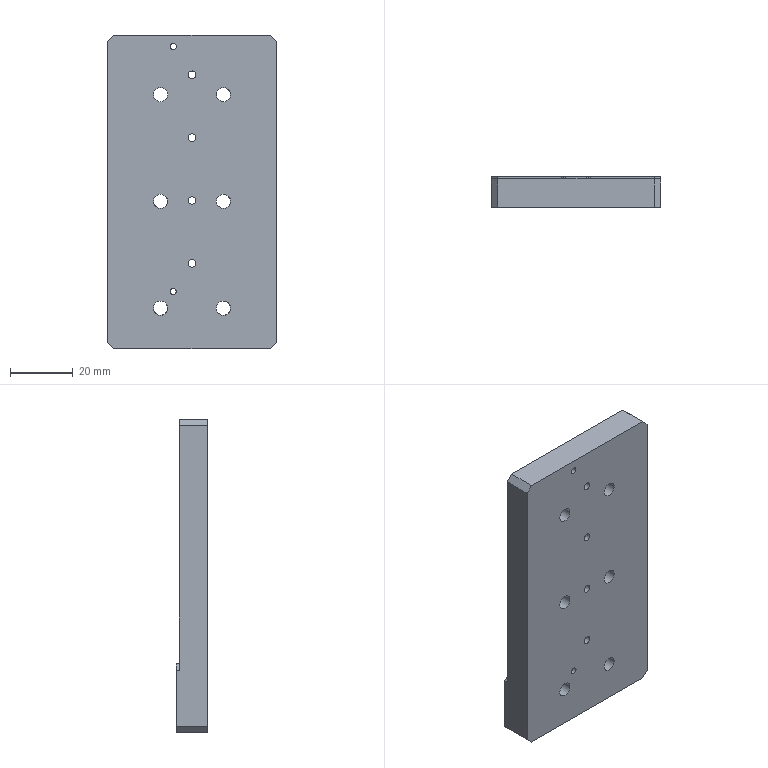CAM job | NX | 3+2 milling, drilling | part box 54 x 10 x 100 mm | stock box 59 x 12 x 105 mm
Tools:
number,name,description,diameter,corner_radius,flute_length,length,flutes
18,D2,平底铣刀-粗,2.0,0.0,50.0,75.0,2
4,D4,平底铣刀-粗,4.0,0.0,25.0,75.0,2
6,D6,平底铣刀-粗,6.0,0.0,25.0,75.0,2
9,D10,平底铣刀-粗,10.0,0.0,35.0,75.0,2
17,D1-J,平底铣刀-粗,0.96,0.0,50.0,75.0,2
19,D2-J,平底铣刀-精,2.0,0.0,50.0,75.0,2
7,D6-J,平底铣刀-精,6.0,0.0,25.0,75.0,2
10,D10-J,平底铣刀-精,10.0,0.0,35.0,75.0,2
1,D80R0.8_FACEMILL,圆鼻刀-粗,80.0,0.8,50.0,75.0,2
1,D80R0.8_FACEMILL-J,圆鼻刀-精,80.0,0.8,50.0,75.0,2
2,D6_CHAMFERTOOL,倒角刀,6.0,0.0,3.0,25.0,2
20,M3X0.5,丝锥,2.5,0.0,35.0,50.0,2
17,ZT2,钻头,2.0,0.0,35.0,50.0,2
12,ZT2.5,钻头,2.5,0.0,35.0,50.0,2
11,ZT4.5,钻头,4.5,0.0,35.0,50.0,2
Operations:
program,operation,operation_type,tool,method,geometry_group,spindle_rpm,surface_speed,feed_per_tooth,feed_cut,feed_plunge,cut_length_mm,path_length_mm,cut_time_min,machine_time_min
B,BOTTOMWALL-FACEONEROUGH_COPY,VolumeBased25DMillingOperation,D80R0.8_FACEMILL,LAYERROUGH-DEPTHK-STEPG,W-B,2800.0,703.696,0.5357,3000.0,100.0,832.776,1479.735,0.2776,0.3423
B,BOTTOMWALL-FACEONEFIN_COPY,VolumeBased25DMillingOperation,D80R0.8_FACEMILL-J,SIDEFINISH-DEPTHK-STEPG,W-B,4000.0,1005.28,0.125,1000.0,100.0,207.998,243.998,0.208,0.2116
B,BOTTOMWALL-LAYERROUGH-MID_COPY,VolumeBased25DMillingOperation,D6,LAYERROUGH-DEPTHK-STEPG,W-B,8000.0,251.32,0.25,4000.0,100.0,2336.776,2441.968,0.5842,0.5947
B,MILLCSK_1,CylinderMilling,D4,METHOD,W-B,8000.0,100.531,0.1125,1800.0,100.0,807.587,1068.388,0.4487,0.4747
B,MILLCSK_2,CylinderMilling,D4,METHOD,W-B,8000.0,100.531,0.1125,1800.0,100.0,473.117,584.517,0.2628,0.274
B,MILLHOLE_1,CylinderMilling,D4,METHOD,W-B,8000.0,100.531,0.0375,600.0,100.0,70.071,352.071,0.1168,0.145
B,MILLHOLE_2,CylinderMilling,D4,METHOD,W-B,8000.0,100.531,0.0375,600.0,100.0,70.071,194.071,0.1168,0.1292
B,MILLCSK_3,CylinderMilling,D2,METHOD,W-B,8000.0,50.266,0.0312,500.0,100.0,75.943,121.643,0.1519,0.1565
B,MILLCSK_4,CylinderMilling,D2,METHOD,W-B,8000.0,50.266,0.0312,500.0,100.0,92.728,137.428,0.1855,0.1899
B,ZLEVEL-SMOOTH-CORNERD2REF6_COPY,ZLevelMilling,D2-J,LAYERFINISH-DEPTHK-STEPG,W-B,8000.0,50.264,0.05,800.0,100.0,174.465,222.28,0.2181,0.2229
B,DRILLCHAMFER_3,Operation,D6_CHAMFERTOOL,METHOD,W-B,8000.0,150.796,0.0625,1000.0,0.0,19.0,149.671,0.019,0.0321
B,MILLCHAMFER_2,PlanarMilling,D6_CHAMFERTOOL,METHOD,W-B,8000.0,150.796,0.0375,600.0,100.0,107.421,504.246,0.179,0.2187
B,PLANARDEBURR6X45L_COPY,SurfaceContour,D6_CHAMFERTOOL,WALLCHAMFER-DEPTH0-STEPG,W-B,6500.0,122.519,0.1154,1500.0,100.0,377.49,466.567,0.2517,0.2606
B,BOTTOMWALL-FINSIDE-MID_COPY,VolumeBased25DMillingOperation,D2-J,SIDEFINISH-DEPTHK-STEPG,W-B,8000.0,50.266,0.0125,200.0,100.0,66.09,205.944,0.3305,0.3444
B,BOTTOMWALL-FINBOTTOM-MID_COPY,VolumeBased25DMillingOperation,D6-J,FINISH-STEPDEPTHOFF,W-B,8000.0,100.528,0.05,800.0,100.0,1546.242,1568.843,1.933,1.935
B,BOTTOMWALL-FINSIDE-MID-SELBOTTOM_COPY,VolumeBased25DMillingOperation,D6-J,SIDEFINISH-DEPTHK-STEPG,W-B,8000.0,100.528,0.05,800.0,100.0,72.512,96.114,0.0906,0.093
B,BOTTOMWALL-FINSIDE-MID_COPY_1,VolumeBased25DMillingOperation,D2-J,SIDEFINISH-DEPTHK-STEPG,W-B,8000.0,50.264,0.0375,600.0,100.0,15.624,38.226,0.026,0.0283
B,ZLEVEL-SMOOTH-CORNERD2REF6_COPY_COPY,ZLevelMilling,D1-J,LAYERFINISH-DEPTHK-STEPG,W-B,12000.0,37.699,0.025,600.0,100.0,309.247,362.878,0.5154,0.5208
A,TOPFACE,FaceMilling,D80R0.8_FACEMILL,SIDEFINISH-DEPTHK-STEPG,W-A,4000.0,1005.31,0.125,1000.0,100.0,194.0,230.0,0.194,0.1976
A,OUTLINE-ROUGH_2,VolumeBased25DMillingOperation,D10,METHOD,W-A,8000.0,251.327,0.3125,5000.0,80.0,5031.881,5080.481,1.006,1.011
A,SPOT-DEPTH0.8,Operation,D6_CHAMFERTOOL,NONE,W-A,8000.0,150.796,0.0312,500.0,90.0,21.6,252.238,0.0432,0.0663
A,THRUHOLE-1-2,Operation,ZT2,NONE,W-A,3000.0,18.85,0.005,30.0,90.0,26.0,171.006,0.8667,0.8812
A,THRUHOLE-M3TAPDRILL,Operation,ZT2.5,NONE,W-A,3000.0,23.562,0.05,300.0,90.0,63.004,229.084,0.21,0.2266
A,THRUHOLE-5-6,Operation,ZT4.5,NONE,W-A,3000.0,42.411,0.025,150.0,90.0,78.0,329.104,0.52,0.5451
A,SOLIDONLY,SurfaceContour,D6_CHAMFERTOOL,METHOD,W-A,8000.0,150.796,0.1875,3000.0,100.0,320.613,356.414,0.1069,0.1105
A,DRILLCHAMFER_1,Operation,D6_CHAMFERTOOL,METHOD,W-A,8000.0,150.796,0.0312,500.0,0.0,8.6,138.258,0.0172,0.0302
A,DRILLCHAMFER_2,Operation,D6_CHAMFERTOOL,METHOD,W-A,8000.0,150.796,0.0312,500.0,0.0,19.0,147.671,0.038,0.0509
A,MILLCHAMFER_1,PlanarMilling,D6_CHAMFERTOOL,METHOD,W-A,8000.0,150.796,0.0312,500.0,100.0,104.118,479.253,0.2082,0.2457
A,THRUHOLE-TAPM3,Operation,M3X0.5,METHOD,W-A,800.0,6.283,0.0003,0.5,90.0,52.0,207.075,104.0,104.016
A,OUTLINE-SEMIFIN_2,VolumeBased25DMillingOperation,D10-J,METHOD,W-A,8000.0,251.327,0.0625,1000.0,100.0,339.688,398.888,0.3397,0.3456